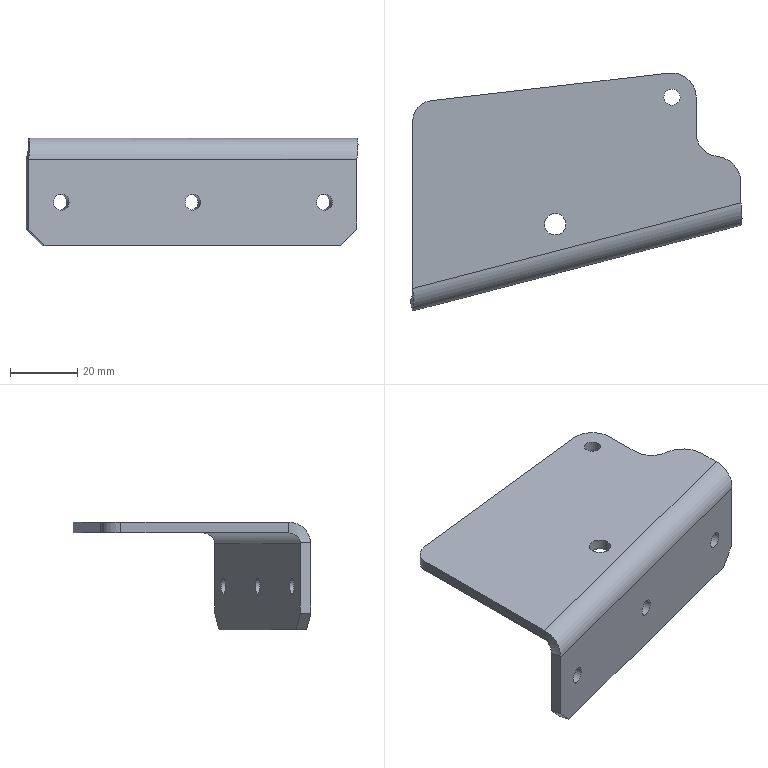Part | NX | features solid 2 | 1 solid | 26 faces | box 98.616 x 70.666 x 32 mm | volume 24079 mm3 | plane 13 | cylinder 11 | spline 2 | commonest cylinder face diameters 4.8 x4 6.4 x2 12 x1 12.8 x1 14 x1 14.4 x1
STEP:
#1=CARTESIAN_POINT('',(-163.637,-50.8,-3.2));
#2=VERTEX_POINT('',#1);
#3=CARTESIAN_POINT('',(-163.637,-56.814,-3.2));
#4=VERTEX_POINT('',#3);
#5=CARTESIAN_POINT('',(-163.637,-32.436,-3.2));
#6=DIRECTION('',(0.,1.,0.));
#7=VECTOR('',#6,1000.);
#8=LINE('',#5,#7);
#9=EDGE_CURVE('',#2,#4,#8,.F.);
#10=ORIENTED_EDGE('',*,*,#9,.T.);
#11=CARTESIAN_POINT('',(-261.143,-82.252,-3.2));
#12=VERTEX_POINT('',#11);
#13=CARTESIAN_POINT('',(-261.143,-82.252,-3.2));
#14=DIRECTION('',(0.9676,0.2524,0.));
#15=VECTOR('',#14,1000.);
#16=LINE('',#13,#15);
#17=EDGE_CURVE('',#4,#12,#16,.F.);
#18=ORIENTED_EDGE('',*,*,#17,.T.);
#19=CARTESIAN_POINT('',(-261.143,-32.436,-3.2));
#20=VERTEX_POINT('',#19);
#21=CARTESIAN_POINT('',(-261.143,-32.436,-3.2));
#22=DIRECTION('',(0.,1.,0.));
#23=VECTOR('',#22,1000.);
#24=LINE('',#21,#23);
#25=EDGE_CURVE('',#12,#20,#24,.T.);
#26=ORIENTED_EDGE('',*,*,#25,.T.);
#27=CARTESIAN_POINT('',(-255.836,-26.476,-3.2));
#28=VERTEX_POINT('',#27);
#29=CARTESIAN_POINT('',(-255.143,-32.436,-3.2));
#30=DIRECTION('',(0.,0.,-1.));
#31=DIRECTION('',(-1.,0.,0.));
#32=AXIS2_PLACEMENT_3D('',#29,#30,#31);
#33=CIRCLE('',#32,6.);
#34=EDGE_CURVE('',#20,#28,#33,.T.);
#35=ORIENTED_EDGE('',*,*,#34,.T.);
#36=CARTESIAN_POINT('',(-184.981,-18.248,-3.2));
#37=VERTEX_POINT('',#36);
#38=CARTESIAN_POINT('',(-255.836,-26.476,-3.2));
#39=DIRECTION('',(0.9933,0.1154,0.));
#40=VECTOR('',#39,1000.);
#41=LINE('',#38,#40);
#42=EDGE_CURVE('',#28,#37,#41,.T.);
#43=ORIENTED_EDGE('',*,*,#42,.T.);
#44=CARTESIAN_POINT('',(-176.95,-25.4,-3.2));
#45=VERTEX_POINT('',#44);
#46=CARTESIAN_POINT('',(-184.15,-25.4,-3.2));
#47=DIRECTION('',(0.,0.,-1.));
#48=DIRECTION('',(-1.,0.,0.));
#49=AXIS2_PLACEMENT_3D('',#46,#47,#48);
#50=CIRCLE('',#49,7.2);
#51=EDGE_CURVE('',#37,#45,#50,.T.);
#52=ORIENTED_EDGE('',*,*,#51,.T.);
#53=CARTESIAN_POINT('',(-176.95,-36.063,-3.2));
#54=VERTEX_POINT('',#53);
#55=CARTESIAN_POINT('',(-176.95,-32.436,-3.2));
#56=DIRECTION('',(0.,1.,0.));
#57=VECTOR('',#56,1000.);
#58=LINE('',#55,#57);
#59=EDGE_CURVE('',#45,#54,#58,.F.);
#60=ORIENTED_EDGE('',*,*,#59,.T.);
#61=CARTESIAN_POINT('',(-170.659,-43.027,-3.2));
#62=VERTEX_POINT('',#61);
#63=CARTESIAN_POINT('',(-169.95,-36.063,-3.2));
#64=DIRECTION('',(0.,0.,1.));
#65=DIRECTION('',(1.,0.,0.));
#66=AXIS2_PLACEMENT_3D('',#63,#64,#65);
#67=CIRCLE('',#66,7.);
#68=EDGE_CURVE('',#54,#62,#67,.T.);
#69=ORIENTED_EDGE('',*,*,#68,.T.);
#70=CARTESIAN_POINT('',(-171.45,-50.8,-3.2));
#71=DIRECTION('',(0.,0.,-1.));
#72=DIRECTION('',(-1.,0.,0.));
#73=AXIS2_PLACEMENT_3D('',#70,#71,#72);
#74=CIRCLE('',#73,7.813);
#75=EDGE_CURVE('',#62,#2,#74,.T.);
#76=ORIENTED_EDGE('',*,*,#75,.T.);
#77=EDGE_LOOP('',(#10,#18,#26,#35,#43,#52,#60,#69,#76));
#78=FACE_BOUND('',#77,.T.);
#79=CARTESIAN_POINT('',(-181.75,-25.4,-3.2));
#80=VERTEX_POINT('',#79);
#81=CARTESIAN_POINT('',(-184.15,-25.4,-3.2));
#82=DIRECTION('',(0.,0.,1.));
#83=DIRECTION('',(1.,0.,0.));
#84=AXIS2_PLACEMENT_3D('',#81,#82,#83);
#85=CIRCLE('',#84,2.4);
#86=EDGE_CURVE('',#80,#80,#85,.T.);
#87=ORIENTED_EDGE('',*,*,#86,.T.);
#88=EDGE_LOOP('',(#87));
#89=FACE_BOUND('',#88,.T.);
#90=CARTESIAN_POINT('',(-222.025,-63.159,-3.2));
#91=VERTEX_POINT('',#90);
#92=CARTESIAN_POINT('',(-218.825,-63.159,-3.2));
#93=DIRECTION('',(0.,0.,-1.));
#94=DIRECTION('',(-1.,0.,0.));
#95=AXIS2_PLACEMENT_3D('',#92,#93,#94);
#96=CIRCLE('',#95,3.2);
#97=EDGE_CURVE('',#91,#91,#96,.F.);
#98=ORIENTED_EDGE('',*,*,#97,.T.);
#99=EDGE_LOOP('',(#98));
#100=FACE_BOUND('',#99,.T.);
#101=CARTESIAN_POINT('',(-255.143,-32.436,-3.2));
#102=DIRECTION('',(0.,0.,-1.));
#103=DIRECTION('',(-1.,0.,0.));
#104=AXIS2_PLACEMENT_3D('',#101,#102,#103);
#105=PLANE('',#104);
#106=ADVANCED_FACE('',(#78,#89,#100),#105,.T.);
#107=CARTESIAN_POINT('',(-261.143,-82.252,0.));
#108=VERTEX_POINT('',#107);
#109=CARTESIAN_POINT('',(-163.637,-56.814,0.));
#110=VERTEX_POINT('',#109);
#111=CARTESIAN_POINT('',(-261.143,-82.252,0.));
#112=DIRECTION('',(0.9676,0.2524,0.));
#113=VECTOR('',#112,1000.);
#114=LINE('',#111,#113);
#115=EDGE_CURVE('',#108,#110,#114,.T.);
#116=ORIENTED_EDGE('',*,*,#115,.T.);
#117=CARTESIAN_POINT('',(-163.637,-50.8,0.));
#118=VERTEX_POINT('',#117);
#119=CARTESIAN_POINT('',(-163.637,-50.8,0.));
#120=DIRECTION('',(0.,-1.,0.));
#121=VECTOR('',#120,1000.);
#122=LINE('',#119,#121);
#123=EDGE_CURVE('',#118,#110,#122,.T.);
#124=ORIENTED_EDGE('',*,*,#123,.F.);
#125=CARTESIAN_POINT('',(-170.659,-43.027,0.));
#126=VERTEX_POINT('',#125);
#127=CARTESIAN_POINT('',(-171.45,-50.8,0.));
#128=DIRECTION('',(0.,0.,-1.));
#129=DIRECTION('',(1.,0.,0.));
#130=AXIS2_PLACEMENT_3D('',#127,#128,#129);
#131=CIRCLE('',#130,7.813);
#132=EDGE_CURVE('',#126,#118,#131,.T.);
#133=ORIENTED_EDGE('',*,*,#132,.F.);
#134=CARTESIAN_POINT('',(-176.95,-36.063,0.));
#135=VERTEX_POINT('',#134);
#136=CARTESIAN_POINT('',(-169.95,-36.063,0.));
#137=DIRECTION('',(0.,0.,1.));
#138=DIRECTION('',(1.,0.,0.));
#139=AXIS2_PLACEMENT_3D('',#136,#137,#138);
#140=CIRCLE('',#139,7.);
#141=EDGE_CURVE('',#135,#126,#140,.T.);
#142=ORIENTED_EDGE('',*,*,#141,.F.);
#143=CARTESIAN_POINT('',(-176.95,-25.4,0.));
#144=VERTEX_POINT('',#143);
#145=CARTESIAN_POINT('',(-176.95,-25.4,0.));
#146=DIRECTION('',(0.,-1.,0.));
#147=VECTOR('',#146,1000.);
#148=LINE('',#145,#147);
#149=EDGE_CURVE('',#144,#135,#148,.T.);
#150=ORIENTED_EDGE('',*,*,#149,.F.);
#151=CARTESIAN_POINT('',(-184.981,-18.248,0.));
#152=VERTEX_POINT('',#151);
#153=CARTESIAN_POINT('',(-184.15,-25.4,0.));
#154=DIRECTION('',(0.,0.,-1.));
#155=DIRECTION('',(1.,0.,0.));
#156=AXIS2_PLACEMENT_3D('',#153,#154,#155);
#157=CIRCLE('',#156,7.2);
#158=EDGE_CURVE('',#152,#144,#157,.T.);
#159=ORIENTED_EDGE('',*,*,#158,.F.);
#160=CARTESIAN_POINT('',(-255.836,-26.476,0.));
#161=VERTEX_POINT('',#160);
#162=CARTESIAN_POINT('',(-255.836,-26.476,0.));
#163=DIRECTION('',(0.9933,0.1154,0.));
#164=VECTOR('',#163,1000.);
#165=LINE('',#162,#164);
#166=EDGE_CURVE('',#161,#152,#165,.T.);
#167=ORIENTED_EDGE('',*,*,#166,.F.);
#168=CARTESIAN_POINT('',(-261.143,-32.436,0.));
#169=VERTEX_POINT('',#168);
#170=CARTESIAN_POINT('',(-255.143,-32.436,0.));
#171=DIRECTION('',(0.,0.,-1.));
#172=DIRECTION('',(1.,0.,0.));
#173=AXIS2_PLACEMENT_3D('',#170,#171,#172);
#174=CIRCLE('',#173,6.);
#175=EDGE_CURVE('',#169,#161,#174,.T.);
#176=ORIENTED_EDGE('',*,*,#175,.F.);
#177=CARTESIAN_POINT('',(-261.143,-88.866,0.));
#178=DIRECTION('',(0.,1.,0.));
#179=VECTOR('',#178,1000.);
#180=LINE('',#177,#179);
#181=EDGE_CURVE('',#108,#169,#180,.T.);
#182=ORIENTED_EDGE('',*,*,#181,.F.);
#183=EDGE_LOOP('',(#116,#124,#133,#142,#150,#159,#167,#176,#182));
#184=FACE_BOUND('',#183,.T.);
#185=CARTESIAN_POINT('',(-181.75,-25.4,0.));
#186=VERTEX_POINT('',#185);
#187=CARTESIAN_POINT('',(-184.15,-25.4,0.));
#188=DIRECTION('',(0.,0.,1.));
#189=DIRECTION('',(1.,0.,0.));
#190=AXIS2_PLACEMENT_3D('',#187,#188,#189);
#191=CIRCLE('',#190,2.4);
#192=EDGE_CURVE('',#186,#186,#191,.T.);
#193=ORIENTED_EDGE('',*,*,#192,.F.);
#194=EDGE_LOOP('',(#193));
#195=FACE_BOUND('',#194,.T.);
#196=CARTESIAN_POINT('',(-222.025,-63.159,0.));
#197=VERTEX_POINT('',#196);
#198=CARTESIAN_POINT('',(-218.825,-63.159,0.));
#199=DIRECTION('',(0.,0.,-1.));
#200=DIRECTION('',(-1.,0.,0.));
#201=AXIS2_PLACEMENT_3D('',#198,#199,#200);
#202=CIRCLE('',#201,3.2);
#203=EDGE_CURVE('',#197,#197,#202,.F.);
#204=ORIENTED_EDGE('',*,*,#203,.F.);
#205=EDGE_LOOP('',(#204));
#206=FACE_BOUND('',#205,.T.);
#207=CARTESIAN_POINT('',(-255.143,-32.436,0.));
#208=DIRECTION('',(0.,0.,-1.));
#209=DIRECTION('',(-1.,0.,0.));
#210=AXIS2_PLACEMENT_3D('',#207,#208,#209);
#211=PLANE('',#210);
#212=ADVANCED_FACE('',(#184,#195,#206),#211,.F.);
#213=CARTESIAN_POINT('',(-163.637,-56.814,0.));
#214=DIRECTION('',(0.,0.,1.));
#215=VECTOR('',#214,1000.);
#216=LINE('',#213,#215);
#217=EDGE_CURVE('',#110,#4,#216,.F.);
#218=ORIENTED_EDGE('',*,*,#217,.T.);
#219=ORIENTED_EDGE('',*,*,#9,.F.);
#220=CARTESIAN_POINT('',(-163.637,-50.8,0.));
#221=DIRECTION('',(0.,0.,1.));
#222=VECTOR('',#221,1000.);
#223=LINE('',#220,#222);
#224=EDGE_CURVE('',#118,#2,#223,.F.);
#225=ORIENTED_EDGE('',*,*,#224,.F.);
#226=ORIENTED_EDGE('',*,*,#123,.T.);
#227=EDGE_LOOP('',(#218,#219,#225,#226));
#228=FACE_BOUND('',#227,.T.);
#229=CARTESIAN_POINT('',(-163.637,-50.8,0.));
#230=DIRECTION('',(1.,0.,0.));
#231=DIRECTION('',(0.,-1.,0.));
#232=AXIS2_PLACEMENT_3D('',#229,#230,#231);
#233=PLANE('',#232);
#234=ADVANCED_FACE('',(#228),#233,.T.);
#235=CARTESIAN_POINT('',(-261.143,-82.252,0.));
#236=DIRECTION('',(0.,0.,1.));
#237=VECTOR('',#236,1000.);
#238=LINE('',#235,#237);
#239=EDGE_CURVE('',#108,#12,#238,.F.);
#240=ORIENTED_EDGE('',*,*,#239,.F.);
#241=ORIENTED_EDGE('',*,*,#181,.T.);
#242=CARTESIAN_POINT('',(-261.143,-32.436,0.));
#243=DIRECTION('',(0.,0.,1.));
#244=VECTOR('',#243,1000.);
#245=LINE('',#242,#244);
#246=EDGE_CURVE('',#169,#20,#245,.F.);
#247=ORIENTED_EDGE('',*,*,#246,.T.);
#248=ORIENTED_EDGE('',*,*,#25,.F.);
#249=EDGE_LOOP('',(#240,#241,#247,#248));
#250=FACE_BOUND('',#249,.T.);
#251=CARTESIAN_POINT('',(-261.143,-88.866,0.));
#252=DIRECTION('',(-1.,0.,0.));
#253=DIRECTION('',(0.,1.,0.));
#254=AXIS2_PLACEMENT_3D('',#251,#252,#253);
#255=PLANE('',#254);
#256=ADVANCED_FACE('',(#250),#255,.T.);
#257=CARTESIAN_POINT('',(-170.659,-43.027,0.));
#258=DIRECTION('',(0.,0.,1.));
#259=VECTOR('',#258,1000.);
#260=LINE('',#257,#259);
#261=EDGE_CURVE('',#126,#62,#260,.F.);
#262=ORIENTED_EDGE('',*,*,#261,.T.);
#263=ORIENTED_EDGE('',*,*,#68,.F.);
#264=CARTESIAN_POINT('',(-176.95,-36.063,0.));
#265=DIRECTION('',(0.,0.,1.));
#266=VECTOR('',#265,1000.);
#267=LINE('',#264,#266);
#268=EDGE_CURVE('',#54,#135,#267,.T.);
#269=ORIENTED_EDGE('',*,*,#268,.T.);
#270=ORIENTED_EDGE('',*,*,#141,.T.);
#271=EDGE_LOOP('',(#262,#263,#269,#270));
#272=FACE_BOUND('',#271,.T.);
#273=CARTESIAN_POINT('',(-169.95,-36.063,0.));
#274=DIRECTION('',(0.,0.,1.));
#275=DIRECTION('',(1.,0.,0.));
#276=AXIS2_PLACEMENT_3D('',#273,#274,#275);
#277=CYLINDRICAL_SURFACE('',#276,7.);
#278=ADVANCED_FACE('',(#272),#277,.F.);
#279=ORIENTED_EDGE('',*,*,#268,.F.);
#280=ORIENTED_EDGE('',*,*,#59,.F.);
#281=CARTESIAN_POINT('',(-176.95,-25.4,0.));
#282=DIRECTION('',(0.,0.,1.));
#283=VECTOR('',#282,1000.);
#284=LINE('',#281,#283);
#285=EDGE_CURVE('',#45,#144,#284,.T.);
#286=ORIENTED_EDGE('',*,*,#285,.T.);
#287=ORIENTED_EDGE('',*,*,#149,.T.);
#288=EDGE_LOOP('',(#279,#280,#286,#287));
#289=FACE_BOUND('',#288,.T.);
#290=CARTESIAN_POINT('',(-176.95,-25.4,0.));
#291=DIRECTION('',(1.,0.,0.));
#292=DIRECTION('',(0.,-1.,0.));
#293=AXIS2_PLACEMENT_3D('',#290,#291,#292);
#294=PLANE('',#293);
#295=ADVANCED_FACE('',(#289),#294,.T.);
#296=ORIENTED_EDGE('',*,*,#285,.F.);
#297=ORIENTED_EDGE('',*,*,#51,.F.);
#298=CARTESIAN_POINT('',(-184.981,-18.248,0.));
#299=DIRECTION('',(0.,0.,1.));
#300=VECTOR('',#299,1000.);
#301=LINE('',#298,#300);
#302=EDGE_CURVE('',#37,#152,#301,.T.);
#303=ORIENTED_EDGE('',*,*,#302,.T.);
#304=ORIENTED_EDGE('',*,*,#158,.T.);
#305=EDGE_LOOP('',(#296,#297,#303,#304));
#306=FACE_BOUND('',#305,.T.);
#307=CARTESIAN_POINT('',(-184.15,-25.4,0.));
#308=DIRECTION('',(0.,0.,-1.));
#309=DIRECTION('',(-1.,0.,0.));
#310=AXIS2_PLACEMENT_3D('',#307,#308,#309);
#311=CYLINDRICAL_SURFACE('',#310,7.2);
#312=ADVANCED_FACE('',(#306),#311,.T.);
#313=ORIENTED_EDGE('',*,*,#302,.F.);
#314=ORIENTED_EDGE('',*,*,#42,.F.);
#315=CARTESIAN_POINT('',(-255.836,-26.476,0.));
#316=DIRECTION('',(0.,0.,1.));
#317=VECTOR('',#316,1000.);
#318=LINE('',#315,#317);
#319=EDGE_CURVE('',#28,#161,#318,.T.);
#320=ORIENTED_EDGE('',*,*,#319,.T.);
#321=ORIENTED_EDGE('',*,*,#166,.T.);
#322=EDGE_LOOP('',(#313,#314,#320,#321));
#323=FACE_BOUND('',#322,.T.);
#324=CARTESIAN_POINT('',(-255.836,-26.476,0.));
#325=DIRECTION('',(-0.1154,0.9933,0.));
#326=DIRECTION('',(0.9933,0.1154,0.));
#327=AXIS2_PLACEMENT_3D('',#324,#325,#326);
#328=PLANE('',#327);
#329=ADVANCED_FACE('',(#323),#328,.T.);
#330=ORIENTED_EDGE('',*,*,#319,.F.);
#331=ORIENTED_EDGE('',*,*,#34,.F.);
#332=ORIENTED_EDGE('',*,*,#246,.F.);
#333=ORIENTED_EDGE('',*,*,#175,.T.);
#334=EDGE_LOOP('',(#330,#331,#332,#333));
#335=FACE_BOUND('',#334,.T.);
#336=CARTESIAN_POINT('',(-255.143,-32.436,0.));
#337=DIRECTION('',(0.,0.,-1.));
#338=DIRECTION('',(-1.,0.,0.));
#339=AXIS2_PLACEMENT_3D('',#336,#337,#338);
#340=CYLINDRICAL_SURFACE('',#339,6.);
#341=ADVANCED_FACE('',(#335),#340,.T.);
#342=ORIENTED_EDGE('',*,*,#132,.T.);
#343=ORIENTED_EDGE('',*,*,#224,.T.);
#344=ORIENTED_EDGE('',*,*,#75,.F.);
#345=ORIENTED_EDGE('',*,*,#261,.F.);
#346=EDGE_LOOP('',(#342,#343,#344,#345));
#347=FACE_BOUND('',#346,.T.);
#348=CARTESIAN_POINT('',(-171.45,-50.8,0.));
#349=DIRECTION('',(0.,0.,-1.));
#350=DIRECTION('',(-1.,0.,0.));
#351=AXIS2_PLACEMENT_3D('',#348,#349,#350);
#352=CYLINDRICAL_SURFACE('',#351,7.813);
#353=ADVANCED_FACE('',(#347),#352,.T.);
#354=ORIENTED_EDGE('',*,*,#192,.T.);
#355=CARTESIAN_POINT('',(-181.75,-25.4,0.));
#356=DIRECTION('',(0.,0.,1.));
#357=VECTOR('',#356,1000.);
#358=LINE('',#355,#357);
#359=EDGE_CURVE('',#186,#80,#358,.F.);
#360=ORIENTED_EDGE('',*,*,#359,.T.);
#361=ORIENTED_EDGE('',*,*,#86,.F.);
#362=ORIENTED_EDGE('',*,*,#359,.F.);
#363=EDGE_LOOP('',(#354,#360,#361,#362));
#364=FACE_BOUND('',#363,.T.);
#365=CARTESIAN_POINT('',(-184.15,-25.4,0.));
#366=DIRECTION('',(0.,0.,1.));
#367=DIRECTION('',(1.,0.,0.));
#368=AXIS2_PLACEMENT_3D('',#365,#366,#367);
#369=CYLINDRICAL_SURFACE('',#368,2.4);
#370=ADVANCED_FACE('',(#364),#369,.F.);
#371=ORIENTED_EDGE('',*,*,#239,.T.);
#372=CARTESIAN_POINT('',(-261.953,-85.763,-6.186));
#373=VERTEX_POINT('',#372);
#374=CARTESIAN_POINT('',(-261.953,-85.763,-6.186));
#375=CARTESIAN_POINT('',(-261.695,-85.639,-5.378));
#376=CARTESIAN_POINT('',(-261.346,-84.783,-3.837));
#377=CARTESIAN_POINT('',(-261.211,-83.106,-3.2));
#378=CARTESIAN_POINT('',(-261.143,-82.252,-3.2));
#379=B_SPLINE_CURVE_WITH_KNOTS('',3,(#374,#375,#376,#377,#378),.UNSPECIFIED.,.F.,.F.,(4,1,4),(0.,0.002534,0.005067),.UNSPECIFIED.);
#380=EDGE_CURVE('',#373,#12,#379,.T.);
#381=ORIENTED_EDGE('',*,*,#380,.F.);
#382=CARTESIAN_POINT('',(-261.147,-88.852,-5.971));
#383=VERTEX_POINT('',#382);
#384=CARTESIAN_POINT('',(-261.147,-88.852,-5.971));
#385=DIRECTION('',(-0.2519,0.9654,-0.06699));
#386=VECTOR('',#385,1000.);
#387=LINE('',#384,#386);
#388=EDGE_CURVE('',#373,#383,#387,.F.);
#389=ORIENTED_EDGE('',*,*,#388,.T.);
#390=CARTESIAN_POINT('',(-261.147,-88.852,-5.971));
#391=CARTESIAN_POINT('',(-260.903,-88.676,-4.357));
#392=CARTESIAN_POINT('',(-260.741,-87.104,-1.274));
#393=CARTESIAN_POINT('',(-261.007,-83.888,0.));
#394=CARTESIAN_POINT('',(-261.143,-82.252,0.));
#395=B_SPLINE_CURVE_WITH_KNOTS('',3,(#390,#391,#392,#393,#394),.UNSPECIFIED.,.F.,.F.,(4,1,4),(0.,0.004857,0.009715),.UNSPECIFIED.);
#396=EDGE_CURVE('',#383,#108,#395,.T.);
#397=ORIENTED_EDGE('',*,*,#396,.T.);
#398=EDGE_LOOP('',(#371,#381,#389,#397));
#399=FACE_BOUND('',#398,.T.);
#400=CARTESIAN_POINT('',(-261.139,-88.883,-5.969));
#401=CARTESIAN_POINT('',(-261.018,-88.796,-5.165));
#402=CARTESIAN_POINT('',(-260.936,-88.56,-4.371));
#403=CARTESIAN_POINT('',(-260.841,-87.821,-2.915));
#404=CARTESIAN_POINT('',(-260.828,-87.318,-2.253));
#405=CARTESIAN_POINT('',(-260.856,-86.109,-1.152));
#406=CARTESIAN_POINT('',(-260.897,-85.403,-0.7131));
#407=CARTESIAN_POINT('',(-261.006,-83.882,-0.1213));
#408=CARTESIAN_POINT('',(-261.075,-83.067,0.032));
#409=CARTESIAN_POINT('',(-261.143,-82.252,0.032));
#410=CARTESIAN_POINT('',(-261.147,-88.852,-5.971));
#411=CARTESIAN_POINT('',(-261.026,-88.765,-5.171));
#412=CARTESIAN_POINT('',(-260.943,-88.531,-4.381));
#413=CARTESIAN_POINT('',(-260.848,-87.795,-2.932));
#414=CARTESIAN_POINT('',(-260.835,-87.294,-2.273));
#415=CARTESIAN_POINT('',(-260.861,-86.09,-1.178));
#416=CARTESIAN_POINT('',(-260.9,-85.388,-0.7414));
#417=CARTESIAN_POINT('',(-261.008,-83.874,-0.1525));
#418=CARTESIAN_POINT('',(-261.076,-83.063,0.000003839));
#419=CARTESIAN_POINT('',(-261.143,-82.252,-0.000001169));
#420=CARTESIAN_POINT('',(-261.953,-85.763,-6.186));
#421=CARTESIAN_POINT('',(-261.825,-85.701,-5.785));
#422=CARTESIAN_POINT('',(-261.717,-85.567,-5.391));
#423=CARTESIAN_POINT('',(-261.534,-85.164,-4.666));
#424=CARTESIAN_POINT('',(-261.46,-84.896,-4.337));
#425=CARTESIAN_POINT('',(-261.339,-84.259,-3.789));
#426=CARTESIAN_POINT('',(-261.291,-83.89,-3.571));
#427=CARTESIAN_POINT('',(-261.21,-83.098,-3.276));
#428=CARTESIAN_POINT('',(-261.177,-82.675,-3.2));
#429=CARTESIAN_POINT('',(-261.143,-82.252,-3.2));
#430=CARTESIAN_POINT('',(-261.961,-85.731,-6.188));
#431=CARTESIAN_POINT('',(-261.833,-85.671,-5.792));
#432=CARTESIAN_POINT('',(-261.724,-85.537,-5.401));
#433=CARTESIAN_POINT('',(-261.541,-85.137,-4.684));
#434=CARTESIAN_POINT('',(-261.466,-84.872,-4.357));
#435=CARTESIAN_POINT('',(-261.344,-84.24,-3.815));
#436=CARTESIAN_POINT('',(-261.295,-83.875,-3.599));
#437=CARTESIAN_POINT('',(-261.212,-83.09,-3.308));
#438=CARTESIAN_POINT('',(-261.178,-82.671,-3.232));
#439=CARTESIAN_POINT('',(-261.143,-82.252,-3.232));
#440=B_SPLINE_SURFACE_WITH_KNOTS('',1,3,((#400,#401,#402,#403,#404,#405,#406,#407,#408,#409),(#410,#411,#412,#413,#414,#415,#416,#417,#418,#419),(#420,#421,#422,#423,#424,#425,#426,#427,#428,#429),(#430,#431,#432,#433,#434,#435,#436,#437,#438,#439)),.RULED_SURF.,.F.,.F.,.F.,(2,1,1,2),(4,2,2,2,4),(-0.01,0.,1.,1.01),(0.,0.25,0.5,0.75,1.),.UNSPECIFIED.);
#441=ADVANCED_FACE('',(#399),#440,.F.);
#442=CARTESIAN_POINT('',(-261.951,-85.77,-27.));
#443=VERTEX_POINT('',#442);
#444=CARTESIAN_POINT('',(-261.951,-85.77,-6.4));
#445=VERTEX_POINT('',#444);
#446=CARTESIAN_POINT('',(-261.951,-85.77,-40.));
#447=DIRECTION('',(0.,0.,1.));
#448=VECTOR('',#447,1000.);
#449=LINE('',#446,#448);
#450=EDGE_CURVE('',#443,#445,#449,.T.);
#451=ORIENTED_EDGE('',*,*,#450,.F.);
#452=CARTESIAN_POINT('',(-261.143,-88.866,-27.));
#453=VERTEX_POINT('',#452);
#454=CARTESIAN_POINT('',(-261.143,-88.866,-27.));
#455=DIRECTION('',(-0.2524,0.9676,0.));
#456=VECTOR('',#455,1000.);
#457=LINE('',#454,#456);
#458=EDGE_CURVE('',#443,#453,#457,.F.);
#459=ORIENTED_EDGE('',*,*,#458,.T.);
#460=CARTESIAN_POINT('',(-261.143,-88.866,-6.4));
#461=VERTEX_POINT('',#460);
#462=CARTESIAN_POINT('',(-261.143,-88.866,-40.));
#463=DIRECTION('',(0.,0.,1.));
#464=VECTOR('',#463,1000.);
#465=LINE('',#462,#464);
#466=EDGE_CURVE('',#453,#461,#465,.T.);
#467=ORIENTED_EDGE('',*,*,#466,.T.);
#468=CARTESIAN_POINT('',(-262.759,-82.673,-6.4));
#469=DIRECTION('',(-0.9676,-0.2524,0.));
#470=DIRECTION('',(0.,0.,-1.));
#471=AXIS2_PLACEMENT_3D('',#468,#469,#470);
#472=CIRCLE('',#471,6.4);
#473=EDGE_CURVE('',#461,#383,#472,.T.);
#474=ORIENTED_EDGE('',*,*,#473,.T.);
#475=ORIENTED_EDGE('',*,*,#388,.F.);
#476=CARTESIAN_POINT('',(-262.759,-82.673,-6.4));
#477=DIRECTION('',(0.9676,0.2524,0.));
#478=DIRECTION('',(-0.2524,0.9676,0.));
#479=AXIS2_PLACEMENT_3D('',#476,#477,#478);
#480=CIRCLE('',#479,3.2);
#481=EDGE_CURVE('',#445,#373,#480,.F.);
#482=ORIENTED_EDGE('',*,*,#481,.F.);
#483=EDGE_LOOP('',(#451,#459,#467,#474,#475,#482));
#484=FACE_BOUND('',#483,.T.);
#485=CARTESIAN_POINT('',(-262.759,-82.673,-6.4));
#486=DIRECTION('',(0.9676,0.2524,0.));
#487=DIRECTION('',(-0.2524,0.9676,0.));
#488=AXIS2_PLACEMENT_3D('',#485,#486,#487);
#489=PLANE('',#488);
#490=ADVANCED_FACE('',(#484),#489,.F.);
#491=CARTESIAN_POINT('',(-163.637,-63.428,-27.));
#492=VERTEX_POINT('',#491);
#493=CARTESIAN_POINT('',(-163.637,-63.428,-6.4));
#494=VERTEX_POINT('',#493);
#495=CARTESIAN_POINT('',(-163.637,-63.428,-40.));
#496=DIRECTION('',(0.,0.,1.));
#497=VECTOR('',#496,1000.);
#498=LINE('',#495,#497);
#499=EDGE_CURVE('',#492,#494,#498,.T.);
#500=ORIENTED_EDGE('',*,*,#499,.F.);
#501=CARTESIAN_POINT('',(-164.445,-60.332,-27.));
#502=VERTEX_POINT('',#501);
#503=CARTESIAN_POINT('',(-164.445,-60.332,-27.));
#504=DIRECTION('',(-0.2524,0.9676,0.));
#505=VECTOR('',#504,1000.);
#506=LINE('',#503,#505);
#507=EDGE_CURVE('',#492,#502,#506,.T.);
#508=ORIENTED_EDGE('',*,*,#507,.T.);
#509=CARTESIAN_POINT('',(-164.445,-60.332,-6.4));
#510=VERTEX_POINT('',#509);
#511=CARTESIAN_POINT('',(-164.445,-60.332,-40.));
#512=DIRECTION('',(0.,0.,1.));
#513=VECTOR('',#512,1000.);
#514=LINE('',#511,#513);
#515=EDGE_CURVE('',#502,#510,#514,.T.);
#516=ORIENTED_EDGE('',*,*,#515,.T.);
#517=CARTESIAN_POINT('',(-164.447,-60.325,-6.186));
#518=VERTEX_POINT('',#517);
#519=CARTESIAN_POINT('',(-165.253,-57.236,-6.4));
#520=DIRECTION('',(0.9676,0.2524,0.));
#521=DIRECTION('',(-0.2524,0.9676,0.));
#522=AXIS2_PLACEMENT_3D('',#519,#520,#521);
#523=CIRCLE('',#522,3.2);
#524=EDGE_CURVE('',#510,#518,#523,.F.);
#525=ORIENTED_EDGE('',*,*,#524,.T.);
#526=CARTESIAN_POINT('',(-163.641,-63.415,-5.971));
#527=VERTEX_POINT('',#526);
#528=CARTESIAN_POINT('',(-164.447,-60.325,-6.186));
#529=CARTESIAN_POINT('',(-164.178,-61.355,-6.114));
#530=CARTESIAN_POINT('',(-163.909,-62.385,-6.043));
#531=CARTESIAN_POINT('',(-163.641,-63.415,-5.971));
#532=B_SPLINE_CURVE_WITH_KNOTS('',3,(#528,#529,#530,#531),.UNSPECIFIED.,.F.,.F.,(4,4),(0.,0.0032),.UNSPECIFIED.);
#533=EDGE_CURVE('',#518,#527,#532,.T.);
#534=ORIENTED_EDGE('',*,*,#533,.T.);
#535=CARTESIAN_POINT('',(-165.253,-57.236,-6.4));
#536=DIRECTION('',(-0.9676,-0.2524,0.));
#537=DIRECTION('',(0.,0.,-1.));
#538=AXIS2_PLACEMENT_3D('',#535,#536,#537);
#539=CIRCLE('',#538,6.4);
#540=EDGE_CURVE('',#494,#527,#539,.T.);
#541=ORIENTED_EDGE('',*,*,#540,.F.);
#542=EDGE_LOOP('',(#500,#508,#516,#525,#534,#541));
#543=FACE_BOUND('',#542,.T.);
#544=CARTESIAN_POINT('',(-165.253,-57.236,-6.4));
#545=DIRECTION('',(0.9676,0.2524,0.));
#546=DIRECTION('',(-0.2524,0.9676,0.));
#547=AXIS2_PLACEMENT_3D('',#544,#545,#546);
#548=PLANE('',#547);
#549=ADVANCED_FACE('',(#543),#548,.T.);
#550=ORIENTED_EDGE('',*,*,#533,.F.);
#551=CARTESIAN_POINT('',(-163.637,-56.814,-3.2));
#552=CARTESIAN_POINT('',(-163.704,-57.668,-3.2));
#553=CARTESIAN_POINT('',(-163.84,-59.344,-3.836));
#554=CARTESIAN_POINT('',(-164.189,-60.202,-5.378));
#555=CARTESIAN_POINT('',(-164.447,-60.325,-6.186));
#556=B_SPLINE_CURVE_WITH_KNOTS('',3,(#551,#552,#553,#554,#555),.UNSPECIFIED.,.F.,.F.,(4,1,4),(0.,0.002534,0.005067),.UNSPECIFIED.);
#557=EDGE_CURVE('',#4,#518,#556,.T.);
#558=ORIENTED_EDGE('',*,*,#557,.F.);
#559=ORIENTED_EDGE('',*,*,#217,.F.);
#560=CARTESIAN_POINT('',(-163.637,-56.814,0.));
#561=CARTESIAN_POINT('',(-163.5,-58.451,0.));
#562=CARTESIAN_POINT('',(-163.234,-61.662,-1.27));
#563=CARTESIAN_POINT('',(-163.396,-63.239,-4.357));
#564=CARTESIAN_POINT('',(-163.641,-63.415,-5.971));
#565=B_SPLINE_CURVE_WITH_KNOTS('',3,(#560,#561,#562,#563,#564),.UNSPECIFIED.,.F.,.F.,(4,1,4),(0.,0.004857,0.009715),.UNSPECIFIED.);
#566=EDGE_CURVE('',#110,#527,#565,.T.);
#567=ORIENTED_EDGE('',*,*,#566,.T.);
#568=EDGE_LOOP('',(#550,#558,#559,#567));
#569=FACE_BOUND('',#568,.T.);
#570=CARTESIAN_POINT('',(-163.637,-56.814,0.032));
#571=CARTESIAN_POINT('',(-163.568,-57.629,0.032));
#572=CARTESIAN_POINT('',(-163.499,-58.444,-0.1213));
#573=CARTESIAN_POINT('',(-163.39,-59.965,-0.7131));
#574=CARTESIAN_POINT('',(-163.35,-60.671,-1.152));
#575=CARTESIAN_POINT('',(-163.322,-61.881,-2.253));
#576=CARTESIAN_POINT('',(-163.334,-62.384,-2.915));
#577=CARTESIAN_POINT('',(-163.429,-63.123,-4.371));
#578=CARTESIAN_POINT('',(-163.512,-63.358,-5.165));
#579=CARTESIAN_POINT('',(-163.633,-63.445,-5.969));
#580=CARTESIAN_POINT('',(-163.637,-56.814,0.));
#581=CARTESIAN_POINT('',(-163.569,-57.625,0.));
#582=CARTESIAN_POINT('',(-163.501,-58.436,-0.1525));
#583=CARTESIAN_POINT('',(-163.394,-59.95,-0.7414));
#584=CARTESIAN_POINT('',(-163.355,-60.653,-1.178));
#585=CARTESIAN_POINT('',(-163.328,-61.857,-2.273));
#586=CARTESIAN_POINT('',(-163.341,-62.358,-2.932));
#587=CARTESIAN_POINT('',(-163.437,-63.093,-4.381));
#588=CARTESIAN_POINT('',(-163.52,-63.327,-5.171));
#589=CARTESIAN_POINT('',(-163.641,-63.415,-5.971));
#590=CARTESIAN_POINT('',(-163.637,-56.814,-3.2));
#591=CARTESIAN_POINT('',(-163.67,-57.237,-3.2));
#592=CARTESIAN_POINT('',(-163.704,-57.66,-3.276));
#593=CARTESIAN_POINT('',(-163.785,-58.452,-3.571));
#594=CARTESIAN_POINT('',(-163.832,-58.821,-3.789));
#595=CARTESIAN_POINT('',(-163.954,-59.458,-4.337));
#596=CARTESIAN_POINT('',(-164.028,-59.726,-4.666));
#597=CARTESIAN_POINT('',(-164.21,-60.129,-5.391));
#598=CARTESIAN_POINT('',(-164.319,-60.264,-5.785));
#599=CARTESIAN_POINT('',(-164.447,-60.325,-6.186));
#600=CARTESIAN_POINT('',(-163.637,-56.814,-3.232));
#601=CARTESIAN_POINT('',(-163.671,-57.233,-3.232));
#602=CARTESIAN_POINT('',(-163.706,-57.653,-3.308));
#603=CARTESIAN_POINT('',(-163.789,-58.437,-3.599));
#604=CARTESIAN_POINT('',(-163.837,-58.803,-3.815));
#605=CARTESIAN_POINT('',(-163.96,-59.434,-4.357));
#606=CARTESIAN_POINT('',(-164.035,-59.7,-4.684));
#607=CARTESIAN_POINT('',(-164.218,-60.099,-5.401));
#608=CARTESIAN_POINT('',(-164.327,-60.233,-5.792));
#609=CARTESIAN_POINT('',(-164.455,-60.294,-6.188));
#610=B_SPLINE_SURFACE_WITH_KNOTS('',1,3,((#570,#571,#572,#573,#574,#575,#576,#577,#578,#579),(#580,#581,#582,#583,#584,#585,#586,#587,#588,#589),(#590,#591,#592,#593,#594,#595,#596,#597,#598,#599),(#600,#601,#602,#603,#604,#605,#606,#607,#608,#609)),.RULED_SURF.,.F.,.F.,.F.,(2,1,1,2),(4,2,2,2,4),(-0.01,0.,1.,1.01),(0.,0.25,0.5,0.75,1.),.UNSPECIFIED.);
#611=ADVANCED_FACE('',(#569),#610,.F.);
#612=ORIENTED_EDGE('',*,*,#566,.F.);
#613=ORIENTED_EDGE('',*,*,#115,.F.);
#614=ORIENTED_EDGE('',*,*,#396,.F.);
#615=ORIENTED_EDGE('',*,*,#473,.F.);
#616=CARTESIAN_POINT('',(-261.143,-88.866,-6.4));
#617=DIRECTION('',(0.9676,0.2524,0.));
#618=VECTOR('',#617,1000.);
#619=LINE('',#616,#618);
#620=EDGE_CURVE('',#461,#494,#619,.T.);
#621=ORIENTED_EDGE('',*,*,#620,.T.);
#622=ORIENTED_EDGE('',*,*,#540,.T.);
#623=EDGE_LOOP('',(#612,#613,#614,#615,#621,#622));
#624=FACE_BOUND('',#623,.T.);
#625=CARTESIAN_POINT('',(-261.143,-82.252,-6.4));
#626=DIRECTION('',(0.9676,0.2524,0.));
#627=DIRECTION('',(0.,0.,-1.));
#628=AXIS2_PLACEMENT_3D('',#625,#626,#627);
#629=CYLINDRICAL_SURFACE('',#628,6.4);
#630=ADVANCED_FACE('',(#624),#629,.T.);
#631=ORIENTED_EDGE('',*,*,#557,.T.);
#632=ORIENTED_EDGE('',*,*,#524,.F.);
#633=CARTESIAN_POINT('',(-261.951,-85.77,-6.4));
#634=DIRECTION('',(0.9676,0.2524,0.));
#635=VECTOR('',#634,1000.);
#636=LINE('',#633,#635);
#637=EDGE_CURVE('',#445,#510,#636,.T.);
#638=ORIENTED_EDGE('',*,*,#637,.F.);
#639=ORIENTED_EDGE('',*,*,#481,.T.);
#640=ORIENTED_EDGE('',*,*,#380,.T.);
#641=ORIENTED_EDGE('',*,*,#17,.F.);
#642=EDGE_LOOP('',(#631,#632,#638,#639,#640,#641));
#643=FACE_BOUND('',#642,.T.);
#644=CARTESIAN_POINT('',(-261.143,-82.252,-6.4));
#645=DIRECTION('',(0.9676,0.2524,0.));
#646=DIRECTION('',(0.,0.,-1.));
#647=AXIS2_PLACEMENT_3D('',#644,#645,#646);
#648=CYLINDRICAL_SURFACE('',#647,3.2);
#649=ADVANCED_FACE('',(#643),#648,.F.);
#650=CARTESIAN_POINT('',(-168.475,-64.691,-32.));
#651=VERTEX_POINT('',#650);
#652=CARTESIAN_POINT('',(-256.305,-87.604,-32.));
#653=VERTEX_POINT('',#652);
#654=CARTESIAN_POINT('',(-163.637,-63.428,-32.));
#655=DIRECTION('',(0.9676,0.2524,0.));
#656=VECTOR('',#655,1000.);
#657=LINE('',#654,#656);
#658=EDGE_CURVE('',#651,#653,#657,.F.);
#659=ORIENTED_EDGE('',*,*,#658,.T.);
#660=CARTESIAN_POINT('',(-257.113,-84.507,-32.));
#661=VERTEX_POINT('',#660);
#662=CARTESIAN_POINT('',(-257.113,-84.507,-32.));
#663=DIRECTION('',(0.2524,-0.9676,0.));
#664=VECTOR('',#663,1000.);
#665=LINE('',#662,#664);
#666=EDGE_CURVE('',#653,#661,#665,.F.);
#667=ORIENTED_EDGE('',*,*,#666,.T.);
#668=CARTESIAN_POINT('',(-169.283,-61.594,-32.));
#669=VERTEX_POINT('',#668);
#670=CARTESIAN_POINT('',(-164.445,-60.332,-32.));
#671=DIRECTION('',(-0.9676,-0.2524,0.));
#672=VECTOR('',#671,1000.);
#673=LINE('',#670,#672);
#674=EDGE_CURVE('',#661,#669,#673,.F.);
#675=ORIENTED_EDGE('',*,*,#674,.T.);
#676=CARTESIAN_POINT('',(-168.475,-64.691,-32.));
#677=DIRECTION('',(-0.2524,0.9676,0.));
#678=VECTOR('',#677,1000.);
#679=LINE('',#676,#678);
#680=EDGE_CURVE('',#669,#651,#679,.F.);
#681=ORIENTED_EDGE('',*,*,#680,.T.);
#682=EDGE_LOOP('',(#659,#667,#675,#681));
#683=FACE_BOUND('',#682,.T.);
#684=CARTESIAN_POINT('',(-163.637,-63.428,-32.));
#685=DIRECTION('',(0.,0.,-1.));
#686=DIRECTION('',(-0.9676,-0.2524,0.));
#687=AXIS2_PLACEMENT_3D('',#684,#685,#686);
#688=PLANE('',#687);
#689=ADVANCED_FACE('',(#683),#688,.T.);
#690=CARTESIAN_POINT('',(-214.712,-76.753,-19.05));
#691=VERTEX_POINT('',#690);
#692=CARTESIAN_POINT('',(-212.39,-76.147,-19.05));
#693=DIRECTION('',(-0.2524,0.9676,0.));
#694=DIRECTION('',(-0.9676,-0.2524,0.));
#695=AXIS2_PLACEMENT_3D('',#692,#693,#694);
#696=CIRCLE('',#695,2.4);
#697=EDGE_CURVE('',#691,#691,#696,.T.);
#698=ORIENTED_EDGE('',*,*,#697,.T.);
#699=EDGE_LOOP('',(#698));
#700=FACE_BOUND('',#699,.T.);
#701=CARTESIAN_POINT('',(-175.635,-66.559,-19.05));
#702=VERTEX_POINT('',#701);
#703=CARTESIAN_POINT('',(-173.313,-65.953,-19.05));
#704=DIRECTION('',(-0.2524,0.9676,0.));
#705=DIRECTION('',(-0.9676,-0.2524,0.));
#706=AXIS2_PLACEMENT_3D('',#703,#704,#705);
#707=CIRCLE('',#706,2.4);
#708=EDGE_CURVE('',#702,#702,#707,.T.);
#709=ORIENTED_EDGE('',*,*,#708,.T.);
#710=EDGE_LOOP('',(#709));
#711=FACE_BOUND('',#710,.T.);
#712=CARTESIAN_POINT('',(-253.79,-86.947,-19.05));
#713=VERTEX_POINT('',#712);
#714=CARTESIAN_POINT('',(-251.467,-86.342,-19.05));
#715=DIRECTION('',(-0.2524,0.9676,0.));
#716=DIRECTION('',(-0.9676,-0.2524,0.));
#717=AXIS2_PLACEMENT_3D('',#714,#715,#716);
#718=CIRCLE('',#717,2.4);
#719=EDGE_CURVE('',#713,#713,#718,.T.);
#720=ORIENTED_EDGE('',*,*,#719,.T.);
#721=EDGE_LOOP('',(#720));
#722=FACE_BOUND('',#721,.T.);
#723=ORIENTED_EDGE('',*,*,#466,.F.);
#724=CARTESIAN_POINT('',(-256.305,-87.604,-32.));
#725=DIRECTION('',(0.6842,0.1785,-0.7071));
#726=VECTOR('',#725,1000.);
#727=LINE('',#724,#726);
#728=EDGE_CURVE('',#453,#653,#727,.T.);
#729=ORIENTED_EDGE('',*,*,#728,.T.);
#730=ORIENTED_EDGE('',*,*,#658,.F.);
#731=CARTESIAN_POINT('',(-163.637,-63.428,-27.));
#732=DIRECTION('',(-0.6842,-0.1785,-0.7071));
#733=VECTOR('',#732,1000.);
#734=LINE('',#731,#733);
#735=EDGE_CURVE('',#651,#492,#734,.F.);
#736=ORIENTED_EDGE('',*,*,#735,.T.);
#737=ORIENTED_EDGE('',*,*,#499,.T.);
#738=ORIENTED_EDGE('',*,*,#620,.F.);
#739=EDGE_LOOP('',(#723,#729,#730,#736,#737,#738));
#740=FACE_BOUND('',#739,.T.);
#741=CARTESIAN_POINT('',(-163.637,-63.428,-40.));
#742=DIRECTION('',(-0.2524,0.9676,0.));
#743=DIRECTION('',(-0.9676,-0.2524,0.));
#744=AXIS2_PLACEMENT_3D('',#741,#742,#743);
#745=PLANE('',#744);
#746=ADVANCED_FACE('',(#700,#711,#722,#740),#745,.F.);
#747=CARTESIAN_POINT('',(-215.52,-73.657,-19.05));
#748=VERTEX_POINT('',#747);
#749=CARTESIAN_POINT('',(-213.198,-73.051,-19.05));
#750=DIRECTION('',(-0.2524,0.9676,0.));
#751=DIRECTION('',(-0.9676,-0.2524,0.));
#752=AXIS2_PLACEMENT_3D('',#749,#750,#751);
#753=CIRCLE('',#752,2.4);
#754=EDGE_CURVE('',#748,#748,#753,.T.);
#755=ORIENTED_EDGE('',*,*,#754,.F.);
#756=EDGE_LOOP('',(#755));
#757=FACE_BOUND('',#756,.T.);
#758=CARTESIAN_POINT('',(-176.443,-63.462,-19.05));
#759=VERTEX_POINT('',#758);
#760=CARTESIAN_POINT('',(-174.121,-62.856,-19.05));
#761=DIRECTION('',(-0.2524,0.9676,0.));
#762=DIRECTION('',(-0.9676,-0.2524,0.));
#763=AXIS2_PLACEMENT_3D('',#760,#761,#762);
#764=CIRCLE('',#763,2.4);
#765=EDGE_CURVE('',#759,#759,#764,.T.);
#766=ORIENTED_EDGE('',*,*,#765,.F.);
#767=EDGE_LOOP('',(#766));
#768=FACE_BOUND('',#767,.T.);
#769=CARTESIAN_POINT('',(-254.597,-83.851,-19.05));
#770=VERTEX_POINT('',#769);
#771=CARTESIAN_POINT('',(-252.275,-83.245,-19.05));
#772=DIRECTION('',(-0.2524,0.9676,0.));
#773=DIRECTION('',(-0.9676,-0.2524,0.));
#774=AXIS2_PLACEMENT_3D('',#771,#772,#773);
#775=CIRCLE('',#774,2.4);
#776=EDGE_CURVE('',#770,#770,#775,.T.);
#777=ORIENTED_EDGE('',*,*,#776,.F.);
#778=EDGE_LOOP('',(#777));
#779=FACE_BOUND('',#778,.T.);
#780=ORIENTED_EDGE('',*,*,#674,.F.);
#781=CARTESIAN_POINT('',(-206.908,-71.41,-83.885));
#782=DIRECTION('',(-0.6842,-0.1785,0.7071));
#783=VECTOR('',#782,1000.);
#784=LINE('',#781,#783);
#785=EDGE_CURVE('',#661,#443,#784,.T.);
#786=ORIENTED_EDGE('',*,*,#785,.T.);
#787=ORIENTED_EDGE('',*,*,#450,.T.);
#788=ORIENTED_EDGE('',*,*,#637,.T.);
#789=ORIENTED_EDGE('',*,*,#515,.F.);
#790=CARTESIAN_POINT('',(-170.734,-61.973,-33.5));
#791=DIRECTION('',(0.6842,0.1785,0.7071));
#792=VECTOR('',#791,1000.);
#793=LINE('',#790,#792);
#794=EDGE_CURVE('',#502,#669,#793,.F.);
#795=ORIENTED_EDGE('',*,*,#794,.T.);
#796=EDGE_LOOP('',(#780,#786,#787,#788,#789,#795));
#797=FACE_BOUND('',#796,.T.);
#798=CARTESIAN_POINT('',(-164.445,-60.332,-40.));
#799=DIRECTION('',(-0.2524,0.9676,0.));
#800=DIRECTION('',(-0.9676,-0.2524,0.));
#801=AXIS2_PLACEMENT_3D('',#798,#799,#800);
#802=PLANE('',#801);
#803=ADVANCED_FACE('',(#757,#768,#779,#797),#802,.T.);
#804=ORIENTED_EDGE('',*,*,#776,.T.);
#805=EDGE_LOOP('',(#804));
#806=FACE_BOUND('',#805,.T.);
#807=ORIENTED_EDGE('',*,*,#719,.F.);
#808=EDGE_LOOP('',(#807));
#809=FACE_BOUND('',#808,.T.);
#810=CARTESIAN_POINT('',(-251.467,-86.342,-19.05));
#811=DIRECTION('',(-0.2524,0.9676,0.));
#812=DIRECTION('',(-0.9676,-0.2524,0.));
#813=AXIS2_PLACEMENT_3D('',#810,#811,#812);
#814=CYLINDRICAL_SURFACE('',#813,2.4);
#815=ADVANCED_FACE('',(#806,#809),#814,.F.);
#816=ORIENTED_EDGE('',*,*,#765,.T.);
#817=EDGE_LOOP('',(#816));
#818=FACE_BOUND('',#817,.T.);
#819=ORIENTED_EDGE('',*,*,#708,.F.);
#820=EDGE_LOOP('',(#819));
#821=FACE_BOUND('',#820,.T.);
#822=CARTESIAN_POINT('',(-173.313,-65.953,-19.05));
#823=DIRECTION('',(-0.2524,0.9676,0.));
#824=DIRECTION('',(-0.9676,-0.2524,0.));
#825=AXIS2_PLACEMENT_3D('',#822,#823,#824);
#826=CYLINDRICAL_SURFACE('',#825,2.4);
#827=ADVANCED_FACE('',(#818,#821),#826,.F.);
#828=ORIENTED_EDGE('',*,*,#754,.T.);
#829=EDGE_LOOP('',(#828));
#830=FACE_BOUND('',#829,.T.);
#831=ORIENTED_EDGE('',*,*,#697,.F.);
#832=EDGE_LOOP('',(#831));
#833=FACE_BOUND('',#832,.T.);
#834=CARTESIAN_POINT('',(-212.39,-76.147,-19.05));
#835=DIRECTION('',(-0.2524,0.9676,0.));
#836=DIRECTION('',(-0.9676,-0.2524,0.));
#837=AXIS2_PLACEMENT_3D('',#834,#835,#836);
#838=CYLINDRICAL_SURFACE('',#837,2.4);
#839=ADVANCED_FACE('',(#830,#833),#838,.F.);
#840=ORIENTED_EDGE('',*,*,#97,.F.);
#841=EDGE_LOOP('',(#840));
#842=FACE_BOUND('',#841,.T.);
#843=ORIENTED_EDGE('',*,*,#203,.T.);
#844=EDGE_LOOP('',(#843));
#845=FACE_BOUND('',#844,.T.);
#846=CARTESIAN_POINT('',(-218.825,-63.159,16.35));
#847=DIRECTION('',(0.,0.,-1.));
#848=DIRECTION('',(0.,1.,0.));
#849=AXIS2_PLACEMENT_3D('',#846,#847,#848);
#850=CYLINDRICAL_SURFACE('',#849,3.2);
#851=ADVANCED_FACE('',(#842,#845),#850,.F.);
#852=ORIENTED_EDGE('',*,*,#728,.F.);
#853=ORIENTED_EDGE('',*,*,#458,.F.);
#854=ORIENTED_EDGE('',*,*,#785,.F.);
#855=ORIENTED_EDGE('',*,*,#666,.F.);
#856=EDGE_LOOP('',(#852,#853,#854,#855));
#857=FACE_BOUND('',#856,.T.);
#858=CARTESIAN_POINT('',(-256.305,-87.604,-32.));
#859=DIRECTION('',(-0.6842,-0.1785,-0.7071));
#860=DIRECTION('',(0.2524,-0.9676,0.));
#861=AXIS2_PLACEMENT_3D('',#858,#859,#860);
#862=PLANE('',#861);
#863=ADVANCED_FACE('',(#857),#862,.T.);
#864=ORIENTED_EDGE('',*,*,#735,.F.);
#865=ORIENTED_EDGE('',*,*,#680,.F.);
#866=ORIENTED_EDGE('',*,*,#794,.F.);
#867=ORIENTED_EDGE('',*,*,#507,.F.);
#868=EDGE_LOOP('',(#864,#865,#866,#867));
#869=FACE_BOUND('',#868,.T.);
#870=CARTESIAN_POINT('',(-165.253,-57.236,-27.));
#871=DIRECTION('',(-0.6842,-0.1785,0.7071));
#872=DIRECTION('',(-0.2524,0.9676,0.));
#873=AXIS2_PLACEMENT_3D('',#870,#871,#872);
#874=PLANE('',#873);
#875=ADVANCED_FACE('',(#869),#874,.F.);
#876=CLOSED_SHELL('',(#106,#212,#234,#256,#278,#295,#312,#329,#341,#353,#370,#441,#490,#549,#611,#630,#649,#689,#746,#803,#815,#827,#839,#851,#863,#875));
#877=MANIFOLD_SOLID_BREP('',#876);
#878=(LENGTH_UNIT()NAMED_UNIT(*)SI_UNIT(.MILLI.,.METRE.));
#879=UNCERTAINTY_MEASURE_WITH_UNIT(LENGTH_MEASURE(0.0508),#878,'','');
#880=(NAMED_UNIT(*)PLANE_ANGLE_UNIT()SI_UNIT($,.RADIAN.));
#881=(NAMED_UNIT(*)SI_UNIT($,.STERADIAN.)SOLID_ANGLE_UNIT());
#882=(GEOMETRIC_REPRESENTATION_CONTEXT(3)GLOBAL_UNCERTAINTY_ASSIGNED_CONTEXT((#879))GLOBAL_UNIT_ASSIGNED_CONTEXT((#878,#880,#881))REPRESENTATION_CONTEXT('',''));
#883=ADVANCED_BREP_SHAPE_REPRESENTATION('',(#877),#882);